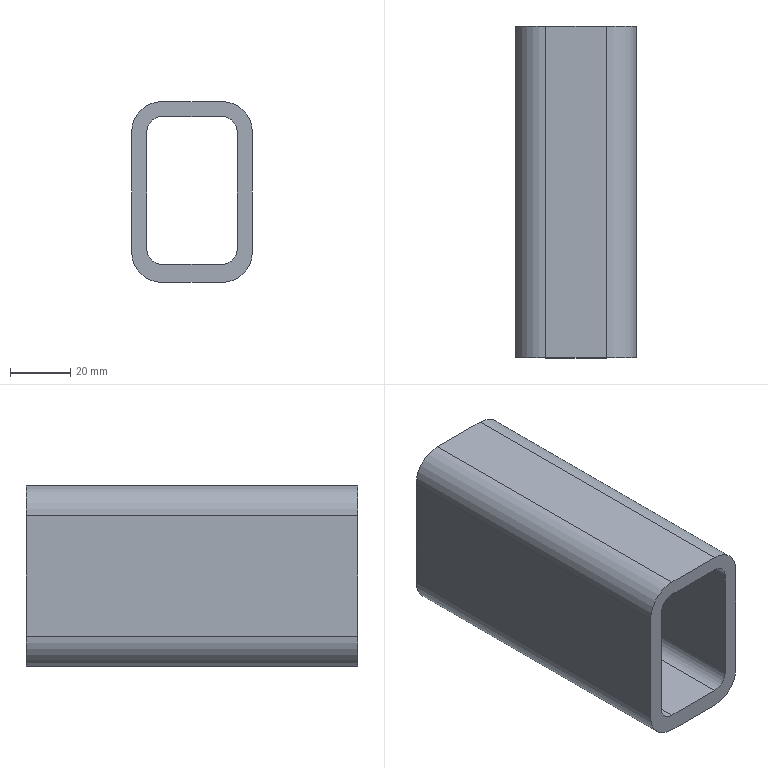Part | STEP file | frame inner longitudinal beam 2--000.001--20240926 | 1 solid | 18 faces | box 40 x 110 x 60 mm | volume 95218 mm3 | plane 10 | cylinder 8 | commonest cylinder face diameters 10 x4 20 x4
STEP:
#1=CARTESIAN_POINT('',(0.,0.,0.));
#2=DIRECTION('',(0.,0.,1.));
#3=DIRECTION('',(1.,0.,0.));
#4=AXIS2_PLACEMENT_3D('',#1,#2,#3);
#5=CARTESIAN_POINT('',(-30.,-995.,50.));
#6=VERTEX_POINT('',#5);
#7=CARTESIAN_POINT('',(-30.,-885.,50.));
#8=VERTEX_POINT('',#7);
#9=CARTESIAN_POINT('',(-30.,490.173,50.));
#10=DIRECTION('',(0.,1.,0.));
#11=VECTOR('',#10,1.);
#12=LINE('',#9,#11);
#13=CARTESIAN_POINT('',(-30.,490.173,40.));
#14=DIRECTION('',(0.,1.,0.));
#15=DIRECTION('',(0.,0.,-1.));
#16=AXIS2_PLACEMENT_3D('',#13,#14,#15);
#17=CYLINDRICAL_SURFACE('',#16,10.);
#18=CARTESIAN_POINT('',(3.142,0.));
#19=DIRECTION('',(0.,1.));
#20=VECTOR('',#19,1.);
#21=LINE('',#18,#20);
#22=(GEOMETRIC_REPRESENTATION_CONTEXT(2)PARAMETRIC_REPRESENTATION_CONTEXT()REPRESENTATION_CONTEXT('',''));
#23=DEFINITIONAL_REPRESENTATION('',(#21),#22);
#24=PCURVE('',#17,#23);
#25=CARTESIAN_POINT('',(-40.,490.173,50.));
#26=DIRECTION('',(0.,0.,-1.));
#27=DIRECTION('',(0.,-1.,0.));
#28=AXIS2_PLACEMENT_3D('',#25,#26,#27);
#29=PLANE('',#28);
#30=CARTESIAN_POINT('',(0.,-10.));
#31=DIRECTION('',(-1.,0.));
#32=VECTOR('',#31,1.);
#33=LINE('',#30,#32);
#34=(GEOMETRIC_REPRESENTATION_CONTEXT(2)PARAMETRIC_REPRESENTATION_CONTEXT()REPRESENTATION_CONTEXT('',''));
#35=DEFINITIONAL_REPRESENTATION('',(#33),#34);
#36=PCURVE('',#29,#35);
#37=SURFACE_CURVE('',#12,(#24,#36),.PCURVE_S1.);
#38=EDGE_CURVE('',#6,#8,#37,.T.);
#39=ORIENTED_EDGE('',*,*,#38,.T.);
#40=CARTESIAN_POINT('',(-40.,-885.,40.));
#41=VERTEX_POINT('',#40);
#42=CARTESIAN_POINT('',(-30.,-885.,40.));
#43=DIRECTION('',(0.,-1.,0.));
#44=DIRECTION('',(0.,0.,1.));
#45=AXIS2_PLACEMENT_3D('',#42,#43,#44);
#46=CIRCLE('',#45,10.);
#47=CARTESIAN_POINT('',(3.142,-1375.173));
#48=DIRECTION('',(-1.,0.));
#49=VECTOR('',#48,1.);
#50=LINE('',#47,#49);
#51=(GEOMETRIC_REPRESENTATION_CONTEXT(2)PARAMETRIC_REPRESENTATION_CONTEXT()REPRESENTATION_CONTEXT('',''));
#52=DEFINITIONAL_REPRESENTATION('',(#50),#51);
#53=PCURVE('',#17,#52);
#54=CARTESIAN_POINT('',(-360.,-885.,20.));
#55=DIRECTION('',(0.,1.,0.));
#56=DIRECTION('',(0.,0.,-1.));
#57=AXIS2_PLACEMENT_3D('',#54,#55,#56);
#58=PLANE('',#57);
#59=CARTESIAN_POINT('',(-30.,-330.));
#60=CARTESIAN_POINT('',(-30.,-312.679));
#61=CARTESIAN_POINT('',(-15.,-321.34));
#62=CARTESIAN_POINT('',(0.,-330.));
#63=CARTESIAN_POINT('',(-15.,-338.66));
#64=CARTESIAN_POINT('',(-30.,-347.321));
#65=CARTESIAN_POINT('',(-30.,-330.));
#66=(BOUNDED_CURVE()B_SPLINE_CURVE(2,(#59,#60,#61,#62,#63,#64,#65),.UNSPECIFIED.,.T.,.F.)B_SPLINE_CURVE_WITH_KNOTS((1,2,2,2,2,1),(-2.094,0.,2.094,4.189,6.283,8.378),.UNSPECIFIED.)CURVE()GEOMETRIC_REPRESENTATION_ITEM()RATIONAL_B_SPLINE_CURVE((1.,0.5,1.,0.5,1.,0.5,1.))REPRESENTATION_ITEM(''));
#67=(GEOMETRIC_REPRESENTATION_CONTEXT(2)PARAMETRIC_REPRESENTATION_CONTEXT()REPRESENTATION_CONTEXT('',''));
#68=DEFINITIONAL_REPRESENTATION('',(#66),#67);
#69=PCURVE('',#58,#68);
#70=SURFACE_CURVE('',#46,(#53,#69),.PCURVE_S1.);
#71=EDGE_CURVE('',#8,#41,#70,.T.);
#72=ORIENTED_EDGE('',*,*,#71,.T.);
#73=CARTESIAN_POINT('',(-40.,-995.,40.));
#74=VERTEX_POINT('',#73);
#75=CARTESIAN_POINT('',(-40.,490.173,40.));
#76=DIRECTION('',(0.,-1.,0.));
#77=VECTOR('',#76,1.);
#78=LINE('',#75,#77);
#79=CARTESIAN_POINT('',(1.571,0.));
#80=DIRECTION('',(0.,-1.));
#81=VECTOR('',#80,1.);
#82=LINE('',#79,#81);
#83=(GEOMETRIC_REPRESENTATION_CONTEXT(2)PARAMETRIC_REPRESENTATION_CONTEXT()REPRESENTATION_CONTEXT('',''));
#84=DEFINITIONAL_REPRESENTATION('',(#82),#83);
#85=PCURVE('',#17,#84);
#86=CARTESIAN_POINT('',(-40.,490.173,10.));
#87=DIRECTION('',(1.,0.,0.));
#88=DIRECTION('',(0.,0.9613,-0.2756));
#89=AXIS2_PLACEMENT_3D('',#86,#87,#88);
#90=PLANE('',#89);
#91=CARTESIAN_POINT('',(-8.269,28.838));
#92=DIRECTION('',(-0.9613,-0.2756));
#93=VECTOR('',#92,1.);
#94=LINE('',#91,#93);
#95=(GEOMETRIC_REPRESENTATION_CONTEXT(2)PARAMETRIC_REPRESENTATION_CONTEXT()REPRESENTATION_CONTEXT('',''));
#96=DEFINITIONAL_REPRESENTATION('',(#94),#95);
#97=PCURVE('',#90,#96);
#98=SURFACE_CURVE('',#78,(#85,#97),.PCURVE_S1.);
#99=EDGE_CURVE('',#41,#74,#98,.T.);
#100=ORIENTED_EDGE('',*,*,#99,.T.);
#101=CARTESIAN_POINT('',(-30.,-995.,40.));
#102=DIRECTION('',(0.,-1.,0.));
#103=DIRECTION('',(0.,0.,1.));
#104=AXIS2_PLACEMENT_3D('',#101,#102,#103);
#105=CIRCLE('',#104,10.);
#106=CARTESIAN_POINT('',(3.142,-1485.173));
#107=DIRECTION('',(-1.,0.));
#108=VECTOR('',#107,1.);
#109=LINE('',#106,#108);
#110=(GEOMETRIC_REPRESENTATION_CONTEXT(2)PARAMETRIC_REPRESENTATION_CONTEXT()REPRESENTATION_CONTEXT('',''));
#111=DEFINITIONAL_REPRESENTATION('',(#109),#110);
#112=PCURVE('',#17,#111);
#113=CARTESIAN_POINT('',(-40.,-995.,-13.42));
#114=DIRECTION('',(0.,1.,0.));
#115=DIRECTION('',(0.,0.,-1.));
#116=AXIS2_PLACEMENT_3D('',#113,#114,#115);
#117=PLANE('',#116);
#118=CARTESIAN_POINT('',(-63.42,-10.));
#119=CARTESIAN_POINT('',(-63.42,7.321));
#120=CARTESIAN_POINT('',(-48.42,-1.34));
#121=CARTESIAN_POINT('',(-33.42,-10.));
#122=CARTESIAN_POINT('',(-48.42,-18.66));
#123=CARTESIAN_POINT('',(-63.42,-27.321));
#124=CARTESIAN_POINT('',(-63.42,-10.));
#125=(BOUNDED_CURVE()B_SPLINE_CURVE(2,(#118,#119,#120,#121,#122,#123,#124),.UNSPECIFIED.,.T.,.F.)B_SPLINE_CURVE_WITH_KNOTS((1,2,2,2,2,1),(-2.094,0.,2.094,4.189,6.283,8.378),.UNSPECIFIED.)CURVE()GEOMETRIC_REPRESENTATION_ITEM()RATIONAL_B_SPLINE_CURVE((1.,0.5,1.,0.5,1.,0.5,1.))REPRESENTATION_ITEM(''));
#126=(GEOMETRIC_REPRESENTATION_CONTEXT(2)PARAMETRIC_REPRESENTATION_CONTEXT()REPRESENTATION_CONTEXT('',''));
#127=DEFINITIONAL_REPRESENTATION('',(#125),#126);
#128=PCURVE('',#117,#127);
#129=SURFACE_CURVE('',#105,(#112,#128),.PCURVE_S1.);
#130=EDGE_CURVE('',#6,#74,#129,.T.);
#131=ORIENTED_EDGE('',*,*,#130,.F.);
#132=EDGE_LOOP('',(#39,#72,#100,#131));
#133=FACE_BOUND('',#132,.T.);
#134=ADVANCED_FACE('',(#133),#17,.T.);
#135=CARTESIAN_POINT('',(-40.,-995.,0.));
#136=VERTEX_POINT('',#135);
#137=CARTESIAN_POINT('',(-40.,-885.,0.));
#138=VERTEX_POINT('',#137);
#139=CARTESIAN_POINT('',(-40.,1110.173,0.));
#140=DIRECTION('',(0.,1.,0.));
#141=VECTOR('',#140,1.);
#142=LINE('',#139,#141);
#143=CARTESIAN_POINT('',(-30.,1110.173,0.));
#144=DIRECTION('',(0.,1.,0.));
#145=DIRECTION('',(0.,0.,-1.));
#146=AXIS2_PLACEMENT_3D('',#143,#144,#145);
#147=CYLINDRICAL_SURFACE('',#146,10.);
#148=CARTESIAN_POINT('',(1.571,0.));
#149=DIRECTION('',(0.,1.));
#150=VECTOR('',#149,1.);
#151=LINE('',#148,#150);
#152=(GEOMETRIC_REPRESENTATION_CONTEXT(2)PARAMETRIC_REPRESENTATION_CONTEXT()REPRESENTATION_CONTEXT('',''));
#153=DEFINITIONAL_REPRESENTATION('',(#151),#152);
#154=PCURVE('',#147,#153);
#155=CARTESIAN_POINT('',(598.739,161.283));
#156=DIRECTION('',(0.9613,0.2756));
#157=VECTOR('',#156,1.);
#158=LINE('',#155,#157);
#159=(GEOMETRIC_REPRESENTATION_CONTEXT(2)PARAMETRIC_REPRESENTATION_CONTEXT()REPRESENTATION_CONTEXT('',''));
#160=DEFINITIONAL_REPRESENTATION('',(#158),#159);
#161=PCURVE('',#90,#160);
#162=SURFACE_CURVE('',#142,(#154,#161),.PCURVE_S1.);
#163=EDGE_CURVE('',#136,#138,#162,.T.);
#164=ORIENTED_EDGE('',*,*,#163,.T.);
#165=CARTESIAN_POINT('',(-30.,-885.,-10.));
#166=VERTEX_POINT('',#165);
#167=CARTESIAN_POINT('',(-30.,-885.,0.));
#168=DIRECTION('',(0.,-1.,0.));
#169=DIRECTION('',(0.,0.,1.));
#170=AXIS2_PLACEMENT_3D('',#167,#168,#169);
#171=CIRCLE('',#170,10.);
#172=CARTESIAN_POINT('',(3.142,-1995.173));
#173=DIRECTION('',(-1.,0.));
#174=VECTOR('',#173,1.);
#175=LINE('',#172,#174);
#176=(GEOMETRIC_REPRESENTATION_CONTEXT(2)PARAMETRIC_REPRESENTATION_CONTEXT()REPRESENTATION_CONTEXT('',''));
#177=DEFINITIONAL_REPRESENTATION('',(#175),#176);
#178=PCURVE('',#147,#177);
#179=CARTESIAN_POINT('',(10.,-330.));
#180=CARTESIAN_POINT('',(10.,-312.679));
#181=CARTESIAN_POINT('',(25.,-321.34));
#182=CARTESIAN_POINT('',(40.,-330.));
#183=CARTESIAN_POINT('',(25.,-338.66));
#184=CARTESIAN_POINT('',(10.,-347.321));
#185=CARTESIAN_POINT('',(10.,-330.));
#186=(BOUNDED_CURVE()B_SPLINE_CURVE(2,(#179,#180,#181,#182,#183,#184,#185),.UNSPECIFIED.,.T.,.F.)B_SPLINE_CURVE_WITH_KNOTS((1,2,2,2,2,1),(-2.094,0.,2.094,4.189,6.283,8.378),.UNSPECIFIED.)CURVE()GEOMETRIC_REPRESENTATION_ITEM()RATIONAL_B_SPLINE_CURVE((1.,0.5,1.,0.5,1.,0.5,1.))REPRESENTATION_ITEM(''));
#187=(GEOMETRIC_REPRESENTATION_CONTEXT(2)PARAMETRIC_REPRESENTATION_CONTEXT()REPRESENTATION_CONTEXT('',''));
#188=DEFINITIONAL_REPRESENTATION('',(#186),#187);
#189=PCURVE('',#58,#188);
#190=SURFACE_CURVE('',#171,(#178,#189),.PCURVE_S1.);
#191=EDGE_CURVE('',#138,#166,#190,.T.);
#192=ORIENTED_EDGE('',*,*,#191,.T.);
#193=CARTESIAN_POINT('',(-30.,-995.,-10.));
#194=VERTEX_POINT('',#193);
#195=CARTESIAN_POINT('',(-30.,1110.173,-10.));
#196=DIRECTION('',(0.,-1.,0.));
#197=VECTOR('',#196,1.);
#198=LINE('',#195,#197);
#199=CARTESIAN_POINT('',(0.,0.));
#200=DIRECTION('',(0.,-1.));
#201=VECTOR('',#200,1.);
#202=LINE('',#199,#201);
#203=(GEOMETRIC_REPRESENTATION_CONTEXT(2)PARAMETRIC_REPRESENTATION_CONTEXT()REPRESENTATION_CONTEXT('',''));
#204=DEFINITIONAL_REPRESENTATION('',(#202),#203);
#205=PCURVE('',#147,#204);
#206=CARTESIAN_POINT('',(0.,1110.173,-10.));
#207=DIRECTION('',(0.,0.,1.));
#208=DIRECTION('',(0.,1.,0.));
#209=AXIS2_PLACEMENT_3D('',#206,#207,#208);
#210=PLANE('',#209);
#211=CARTESIAN_POINT('',(0.,30.));
#212=DIRECTION('',(-1.,0.));
#213=VECTOR('',#212,1.);
#214=LINE('',#211,#213);
#215=(GEOMETRIC_REPRESENTATION_CONTEXT(2)PARAMETRIC_REPRESENTATION_CONTEXT()REPRESENTATION_CONTEXT('',''));
#216=DEFINITIONAL_REPRESENTATION('',(#214),#215);
#217=PCURVE('',#210,#216);
#218=SURFACE_CURVE('',#198,(#205,#217),.PCURVE_S1.);
#219=EDGE_CURVE('',#166,#194,#218,.T.);
#220=ORIENTED_EDGE('',*,*,#219,.T.);
#221=CARTESIAN_POINT('',(-30.,-995.,0.));
#222=DIRECTION('',(0.,-1.,0.));
#223=DIRECTION('',(0.,0.,1.));
#224=AXIS2_PLACEMENT_3D('',#221,#222,#223);
#225=CIRCLE('',#224,10.);
#226=CARTESIAN_POINT('',(3.142,-2105.173));
#227=DIRECTION('',(-1.,0.));
#228=VECTOR('',#227,1.);
#229=LINE('',#226,#228);
#230=(GEOMETRIC_REPRESENTATION_CONTEXT(2)PARAMETRIC_REPRESENTATION_CONTEXT()REPRESENTATION_CONTEXT('',''));
#231=DEFINITIONAL_REPRESENTATION('',(#229),#230);
#232=PCURVE('',#147,#231);
#233=CARTESIAN_POINT('',(-23.42,-10.));
#234=CARTESIAN_POINT('',(-23.42,7.321));
#235=CARTESIAN_POINT('',(-8.42,-1.34));
#236=CARTESIAN_POINT('',(6.58,-10.));
#237=CARTESIAN_POINT('',(-8.42,-18.66));
#238=CARTESIAN_POINT('',(-23.42,-27.321));
#239=CARTESIAN_POINT('',(-23.42,-10.));
#240=(BOUNDED_CURVE()B_SPLINE_CURVE(2,(#233,#234,#235,#236,#237,#238,#239),.UNSPECIFIED.,.T.,.F.)B_SPLINE_CURVE_WITH_KNOTS((1,2,2,2,2,1),(-2.094,0.,2.094,4.189,6.283,8.378),.UNSPECIFIED.)CURVE()GEOMETRIC_REPRESENTATION_ITEM()RATIONAL_B_SPLINE_CURVE((1.,0.5,1.,0.5,1.,0.5,1.))REPRESENTATION_ITEM(''));
#241=(GEOMETRIC_REPRESENTATION_CONTEXT(2)PARAMETRIC_REPRESENTATION_CONTEXT()REPRESENTATION_CONTEXT('',''));
#242=DEFINITIONAL_REPRESENTATION('',(#240),#241);
#243=PCURVE('',#117,#242);
#244=SURFACE_CURVE('',#225,(#232,#243),.PCURVE_S1.);
#245=EDGE_CURVE('',#136,#194,#244,.T.);
#246=ORIENTED_EDGE('',*,*,#245,.F.);
#247=EDGE_LOOP('',(#164,#192,#220,#246));
#248=FACE_BOUND('',#247,.T.);
#249=ADVANCED_FACE('',(#248),#147,.T.);
#250=CARTESIAN_POINT('',(-40.,-885.,10.));
#251=DIRECTION('',(0.,0.,1.));
#252=VECTOR('',#251,1.);
#253=LINE('',#250,#252);
#254=CARTESIAN_POINT('',(-1321.901,-379.049));
#255=DIRECTION('',(-0.2756,0.9613));
#256=VECTOR('',#255,1.);
#257=LINE('',#254,#256);
#258=(GEOMETRIC_REPRESENTATION_CONTEXT(2)PARAMETRIC_REPRESENTATION_CONTEXT()REPRESENTATION_CONTEXT('',''));
#259=DEFINITIONAL_REPRESENTATION('',(#257),#258);
#260=PCURVE('',#90,#259);
#261=CARTESIAN_POINT('',(10.,-320.));
#262=DIRECTION('',(-1.,0.));
#263=VECTOR('',#262,1.);
#264=LINE('',#261,#263);
#265=(GEOMETRIC_REPRESENTATION_CONTEXT(2)PARAMETRIC_REPRESENTATION_CONTEXT()REPRESENTATION_CONTEXT('',''));
#266=DEFINITIONAL_REPRESENTATION('',(#264),#265);
#267=PCURVE('',#58,#266);
#268=SURFACE_CURVE('',#253,(#260,#267),.PCURVE_S1.);
#269=EDGE_CURVE('',#138,#41,#268,.T.);
#270=ORIENTED_EDGE('',*,*,#269,.F.);
#271=ORIENTED_EDGE('',*,*,#163,.F.);
#272=CARTESIAN_POINT('',(-40.,-995.,10.));
#273=DIRECTION('',(0.,0.,1.));
#274=VECTOR('',#273,1.);
#275=LINE('',#272,#274);
#276=CARTESIAN_POINT('',(-1427.64,-409.369));
#277=DIRECTION('',(-0.2756,0.9613));
#278=VECTOR('',#277,1.);
#279=LINE('',#276,#278);
#280=(GEOMETRIC_REPRESENTATION_CONTEXT(2)PARAMETRIC_REPRESENTATION_CONTEXT()REPRESENTATION_CONTEXT('',''));
#281=DEFINITIONAL_REPRESENTATION('',(#279),#280);
#282=PCURVE('',#90,#281);
#283=CARTESIAN_POINT('',(-23.42,0.));
#284=DIRECTION('',(-1.,0.));
#285=VECTOR('',#284,1.);
#286=LINE('',#283,#285);
#287=(GEOMETRIC_REPRESENTATION_CONTEXT(2)PARAMETRIC_REPRESENTATION_CONTEXT()REPRESENTATION_CONTEXT('',''));
#288=DEFINITIONAL_REPRESENTATION('',(#286),#287);
#289=PCURVE('',#117,#288);
#290=SURFACE_CURVE('',#275,(#282,#289),.PCURVE_S1.);
#291=EDGE_CURVE('',#136,#74,#290,.T.);
#292=ORIENTED_EDGE('',*,*,#291,.T.);
#293=ORIENTED_EDGE('',*,*,#99,.F.);
#294=EDGE_LOOP('',(#270,#271,#292,#293));
#295=FACE_BOUND('',#294,.T.);
#296=ADVANCED_FACE('',(#295),#90,.F.);
#297=CARTESIAN_POINT('',(-10.,-995.,-10.));
#298=VERTEX_POINT('',#297);
#299=CARTESIAN_POINT('',(-10.,-885.,-10.));
#300=VERTEX_POINT('',#299);
#301=CARTESIAN_POINT('',(-10.,490.173,-10.));
#302=DIRECTION('',(0.,1.,0.));
#303=VECTOR('',#302,1.);
#304=LINE('',#301,#303);
#305=CARTESIAN_POINT('',(-10.,490.173,0.));
#306=DIRECTION('',(0.,1.,0.));
#307=DIRECTION('',(0.,0.,-1.));
#308=AXIS2_PLACEMENT_3D('',#305,#306,#307);
#309=CYLINDRICAL_SURFACE('',#308,10.);
#310=CARTESIAN_POINT('',(6.283,0.));
#311=DIRECTION('',(0.,1.));
#312=VECTOR('',#311,1.);
#313=LINE('',#310,#312);
#314=(GEOMETRIC_REPRESENTATION_CONTEXT(2)PARAMETRIC_REPRESENTATION_CONTEXT()REPRESENTATION_CONTEXT('',''));
#315=DEFINITIONAL_REPRESENTATION('',(#313),#314);
#316=PCURVE('',#309,#315);
#317=CARTESIAN_POINT('',(-620.,10.));
#318=DIRECTION('',(1.,0.));
#319=VECTOR('',#318,1.);
#320=LINE('',#317,#319);
#321=(GEOMETRIC_REPRESENTATION_CONTEXT(2)PARAMETRIC_REPRESENTATION_CONTEXT()REPRESENTATION_CONTEXT('',''));
#322=DEFINITIONAL_REPRESENTATION('',(#320),#321);
#323=PCURVE('',#210,#322);
#324=SURFACE_CURVE('',#304,(#316,#323),.PCURVE_S1.);
#325=EDGE_CURVE('',#298,#300,#324,.T.);
#326=ORIENTED_EDGE('',*,*,#325,.T.);
#327=CARTESIAN_POINT('',(0.,-885.,0.));
#328=VERTEX_POINT('',#327);
#329=CARTESIAN_POINT('',(-10.,-885.,0.));
#330=DIRECTION('',(0.,-1.,0.));
#331=DIRECTION('',(0.,0.,1.));
#332=AXIS2_PLACEMENT_3D('',#329,#330,#331);
#333=CIRCLE('',#332,10.);
#334=CARTESIAN_POINT('',(9.425,-1375.173));
#335=DIRECTION('',(-1.,0.));
#336=VECTOR('',#335,1.);
#337=LINE('',#334,#336);
#338=(GEOMETRIC_REPRESENTATION_CONTEXT(2)PARAMETRIC_REPRESENTATION_CONTEXT()REPRESENTATION_CONTEXT('',''));
#339=DEFINITIONAL_REPRESENTATION('',(#337),#338);
#340=PCURVE('',#309,#339);
#341=CARTESIAN_POINT('',(10.,-350.));
#342=CARTESIAN_POINT('',(10.,-332.679));
#343=CARTESIAN_POINT('',(25.,-341.34));
#344=CARTESIAN_POINT('',(40.,-350.));
#345=CARTESIAN_POINT('',(25.,-358.66));
#346=CARTESIAN_POINT('',(10.,-367.321));
#347=CARTESIAN_POINT('',(10.,-350.));
#348=(BOUNDED_CURVE()B_SPLINE_CURVE(2,(#341,#342,#343,#344,#345,#346,#347),.UNSPECIFIED.,.T.,.F.)B_SPLINE_CURVE_WITH_KNOTS((1,2,2,2,2,1),(-2.094,0.,2.094,4.189,6.283,8.378),.UNSPECIFIED.)CURVE()GEOMETRIC_REPRESENTATION_ITEM()RATIONAL_B_SPLINE_CURVE((1.,0.5,1.,0.5,1.,0.5,1.))REPRESENTATION_ITEM(''));
#349=(GEOMETRIC_REPRESENTATION_CONTEXT(2)PARAMETRIC_REPRESENTATION_CONTEXT()REPRESENTATION_CONTEXT('',''));
#350=DEFINITIONAL_REPRESENTATION('',(#348),#349);
#351=PCURVE('',#58,#350);
#352=SURFACE_CURVE('',#333,(#340,#351),.PCURVE_S1.);
#353=EDGE_CURVE('',#300,#328,#352,.T.);
#354=ORIENTED_EDGE('',*,*,#353,.T.);
#355=CARTESIAN_POINT('',(0.,-995.,0.));
#356=VERTEX_POINT('',#355);
#357=CARTESIAN_POINT('',(0.,490.173,0.));
#358=DIRECTION('',(0.,-1.,0.));
#359=VECTOR('',#358,1.);
#360=LINE('',#357,#359);
#361=CARTESIAN_POINT('',(4.712,0.));
#362=DIRECTION('',(0.,-1.));
#363=VECTOR('',#362,1.);
#364=LINE('',#361,#363);
#365=(GEOMETRIC_REPRESENTATION_CONTEXT(2)PARAMETRIC_REPRESENTATION_CONTEXT()REPRESENTATION_CONTEXT('',''));
#366=DEFINITIONAL_REPRESENTATION('',(#364),#365);
#367=PCURVE('',#309,#366);
#368=CARTESIAN_POINT('',(0.,490.173,50.));
#369=DIRECTION('',(-1.,0.,0.));
#370=DIRECTION('',(0.,-0.9613,0.2756));
#371=AXIS2_PLACEMENT_3D('',#368,#369,#370);
#372=PLANE('',#371);
#373=CARTESIAN_POINT('',(-13.782,-48.063));
#374=DIRECTION('',(0.9613,-0.2756));
#375=VECTOR('',#374,1.);
#376=LINE('',#373,#375);
#377=(GEOMETRIC_REPRESENTATION_CONTEXT(2)PARAMETRIC_REPRESENTATION_CONTEXT()REPRESENTATION_CONTEXT('',''));
#378=DEFINITIONAL_REPRESENTATION('',(#376),#377);
#379=PCURVE('',#372,#378);
#380=SURFACE_CURVE('',#360,(#367,#379),.PCURVE_S1.);
#381=EDGE_CURVE('',#328,#356,#380,.T.);
#382=ORIENTED_EDGE('',*,*,#381,.T.);
#383=CARTESIAN_POINT('',(-10.,-995.,0.));
#384=DIRECTION('',(0.,1.,0.));
#385=DIRECTION('',(0.,0.,1.));
#386=AXIS2_PLACEMENT_3D('',#383,#384,#385);
#387=CIRCLE('',#386,10.);
#388=CARTESIAN_POINT('',(3.142,-1485.173));
#389=DIRECTION('',(1.,0.));
#390=VECTOR('',#389,1.);
#391=LINE('',#388,#390);
#392=(GEOMETRIC_REPRESENTATION_CONTEXT(2)PARAMETRIC_REPRESENTATION_CONTEXT()REPRESENTATION_CONTEXT('',''));
#393=DEFINITIONAL_REPRESENTATION('',(#391),#392);
#394=PCURVE('',#309,#393);
#395=CARTESIAN_POINT('',(-13.42,-30.));
#396=DIRECTION('',(-1.,0.));
#397=AXIS2_PLACEMENT_2D('',#395,#396);
#398=CIRCLE('',#397,10.);
#399=(GEOMETRIC_REPRESENTATION_CONTEXT(2)PARAMETRIC_REPRESENTATION_CONTEXT()REPRESENTATION_CONTEXT('',''));
#400=DEFINITIONAL_REPRESENTATION('',(#398),#399);
#401=PCURVE('',#117,#400);
#402=SURFACE_CURVE('',#387,(#394,#401),.PCURVE_S1.);
#403=EDGE_CURVE('',#356,#298,#402,.T.);
#404=ORIENTED_EDGE('',*,*,#403,.T.);
#405=EDGE_LOOP('',(#326,#354,#382,#404));
#406=FACE_BOUND('',#405,.T.);
#407=ADVANCED_FACE('',(#406),#309,.T.);
#408=CARTESIAN_POINT('',(0.,-885.,-10.));
#409=DIRECTION('',(-1.,0.,0.));
#410=VECTOR('',#409,1.);
#411=LINE('',#408,#410);
#412=CARTESIAN_POINT('',(-1995.173,0.));
#413=DIRECTION('',(0.,1.));
#414=VECTOR('',#413,1.);
#415=LINE('',#412,#414);
#416=(GEOMETRIC_REPRESENTATION_CONTEXT(2)PARAMETRIC_REPRESENTATION_CONTEXT()REPRESENTATION_CONTEXT('',''));
#417=DEFINITIONAL_REPRESENTATION('',(#415),#416);
#418=PCURVE('',#210,#417);
#419=CARTESIAN_POINT('',(30.,-360.));
#420=DIRECTION('',(0.,1.));
#421=VECTOR('',#420,1.);
#422=LINE('',#419,#421);
#423=(GEOMETRIC_REPRESENTATION_CONTEXT(2)PARAMETRIC_REPRESENTATION_CONTEXT()REPRESENTATION_CONTEXT('',''));
#424=DEFINITIONAL_REPRESENTATION('',(#422),#423);
#425=PCURVE('',#58,#424);
#426=SURFACE_CURVE('',#411,(#418,#425),.PCURVE_S1.);
#427=EDGE_CURVE('',#300,#166,#426,.T.);
#428=ORIENTED_EDGE('',*,*,#427,.F.);
#429=ORIENTED_EDGE('',*,*,#325,.F.);
#430=CARTESIAN_POINT('',(-40.,-995.,-10.));
#431=DIRECTION('',(1.,0.,0.));
#432=VECTOR('',#431,1.);
#433=LINE('',#430,#432);
#434=CARTESIAN_POINT('',(-2105.173,40.));
#435=DIRECTION('',(0.,-1.));
#436=VECTOR('',#435,1.);
#437=LINE('',#434,#436);
#438=(GEOMETRIC_REPRESENTATION_CONTEXT(2)PARAMETRIC_REPRESENTATION_CONTEXT()REPRESENTATION_CONTEXT('',''));
#439=DEFINITIONAL_REPRESENTATION('',(#437),#438);
#440=PCURVE('',#210,#439);
#441=CARTESIAN_POINT('',(-3.42,0.));
#442=DIRECTION('',(0.,-1.));
#443=VECTOR('',#442,1.);
#444=LINE('',#441,#443);
#445=(GEOMETRIC_REPRESENTATION_CONTEXT(2)PARAMETRIC_REPRESENTATION_CONTEXT()REPRESENTATION_CONTEXT('',''));
#446=DEFINITIONAL_REPRESENTATION('',(#444),#445);
#447=PCURVE('',#117,#446);
#448=SURFACE_CURVE('',#433,(#440,#447),.PCURVE_S1.);
#449=EDGE_CURVE('',#194,#298,#448,.T.);
#450=ORIENTED_EDGE('',*,*,#449,.F.);
#451=ORIENTED_EDGE('',*,*,#219,.F.);
#452=EDGE_LOOP('',(#428,#429,#450,#451));
#453=FACE_BOUND('',#452,.T.);
#454=ADVANCED_FACE('',(#453),#210,.F.);
#455=CARTESIAN_POINT('',(0.,-995.,40.));
#456=VERTEX_POINT('',#455);
#457=CARTESIAN_POINT('',(0.,-885.,40.));
#458=VERTEX_POINT('',#457);
#459=CARTESIAN_POINT('',(0.,490.173,40.));
#460=DIRECTION('',(0.,1.,0.));
#461=VECTOR('',#460,1.);
#462=LINE('',#459,#461);
#463=CARTESIAN_POINT('',(-10.,490.173,40.));
#464=DIRECTION('',(0.,1.,0.));
#465=DIRECTION('',(0.,0.,-1.));
#466=AXIS2_PLACEMENT_3D('',#463,#464,#465);
#467=CYLINDRICAL_SURFACE('',#466,10.);
#468=CARTESIAN_POINT('',(4.712,0.));
#469=DIRECTION('',(0.,1.));
#470=VECTOR('',#469,1.);
#471=LINE('',#468,#470);
#472=(GEOMETRIC_REPRESENTATION_CONTEXT(2)PARAMETRIC_REPRESENTATION_CONTEXT()REPRESENTATION_CONTEXT('',''));
#473=DEFINITIONAL_REPRESENTATION('',(#471),#472);
#474=PCURVE('',#467,#473);
#475=CARTESIAN_POINT('',(-2.756,-9.613));
#476=DIRECTION('',(-0.9613,0.2756));
#477=VECTOR('',#476,1.);
#478=LINE('',#475,#477);
#479=(GEOMETRIC_REPRESENTATION_CONTEXT(2)PARAMETRIC_REPRESENTATION_CONTEXT()REPRESENTATION_CONTEXT('',''));
#480=DEFINITIONAL_REPRESENTATION('',(#478),#479);
#481=PCURVE('',#372,#480);
#482=SURFACE_CURVE('',#462,(#474,#481),.PCURVE_S1.);
#483=EDGE_CURVE('',#456,#458,#482,.T.);
#484=ORIENTED_EDGE('',*,*,#483,.T.);
#485=CARTESIAN_POINT('',(-10.,-885.,50.));
#486=VERTEX_POINT('',#485);
#487=CARTESIAN_POINT('',(-10.,-885.,40.));
#488=DIRECTION('',(0.,-1.,0.));
#489=DIRECTION('',(0.,0.,1.));
#490=AXIS2_PLACEMENT_3D('',#487,#488,#489);
#491=CIRCLE('',#490,10.);
#492=CARTESIAN_POINT('',(9.425,-1375.173));
#493=DIRECTION('',(-1.,0.));
#494=VECTOR('',#493,1.);
#495=LINE('',#492,#494);
#496=(GEOMETRIC_REPRESENTATION_CONTEXT(2)PARAMETRIC_REPRESENTATION_CONTEXT()REPRESENTATION_CONTEXT('',''));
#497=DEFINITIONAL_REPRESENTATION('',(#495),#496);
#498=PCURVE('',#467,#497);
#499=CARTESIAN_POINT('',(-30.,-350.));
#500=CARTESIAN_POINT('',(-30.,-332.679));
#501=CARTESIAN_POINT('',(-15.,-341.34));
#502=CARTESIAN_POINT('',(0.,-350.));
#503=CARTESIAN_POINT('',(-15.,-358.66));
#504=CARTESIAN_POINT('',(-30.,-367.321));
#505=CARTESIAN_POINT('',(-30.,-350.));
#506=(BOUNDED_CURVE()B_SPLINE_CURVE(2,(#499,#500,#501,#502,#503,#504,#505),.UNSPECIFIED.,.T.,.F.)B_SPLINE_CURVE_WITH_KNOTS((1,2,2,2,2,1),(-2.094,0.,2.094,4.189,6.283,8.378),.UNSPECIFIED.)CURVE()GEOMETRIC_REPRESENTATION_ITEM()RATIONAL_B_SPLINE_CURVE((1.,0.5,1.,0.5,1.,0.5,1.))REPRESENTATION_ITEM(''));
#507=(GEOMETRIC_REPRESENTATION_CONTEXT(2)PARAMETRIC_REPRESENTATION_CONTEXT()REPRESENTATION_CONTEXT('',''));
#508=DEFINITIONAL_REPRESENTATION('',(#506),#507);
#509=PCURVE('',#58,#508);
#510=SURFACE_CURVE('',#491,(#498,#509),.PCURVE_S1.);
#511=EDGE_CURVE('',#458,#486,#510,.T.);
#512=ORIENTED_EDGE('',*,*,#511,.T.);
#513=CARTESIAN_POINT('',(-10.,-995.,50.));
#514=VERTEX_POINT('',#513);
#515=CARTESIAN_POINT('',(-10.,490.173,50.));
#516=DIRECTION('',(0.,-1.,0.));
#517=VECTOR('',#516,1.);
#518=LINE('',#515,#517);
#519=CARTESIAN_POINT('',(3.142,0.));
#520=DIRECTION('',(0.,-1.));
#521=VECTOR('',#520,1.);
#522=LINE('',#519,#521);
#523=(GEOMETRIC_REPRESENTATION_CONTEXT(2)PARAMETRIC_REPRESENTATION_CONTEXT()REPRESENTATION_CONTEXT('',''));
#524=DEFINITIONAL_REPRESENTATION('',(#522),#523);
#525=PCURVE('',#467,#524);
#526=CARTESIAN_POINT('',(0.,-30.));
#527=DIRECTION('',(1.,0.));
#528=VECTOR('',#527,1.);
#529=LINE('',#526,#528);
#530=(GEOMETRIC_REPRESENTATION_CONTEXT(2)PARAMETRIC_REPRESENTATION_CONTEXT()REPRESENTATION_CONTEXT('',''));
#531=DEFINITIONAL_REPRESENTATION('',(#529),#530);
#532=PCURVE('',#29,#531);
#533=SURFACE_CURVE('',#518,(#525,#532),.PCURVE_S1.);
#534=EDGE_CURVE('',#486,#514,#533,.T.);
#535=ORIENTED_EDGE('',*,*,#534,.T.);
#536=CARTESIAN_POINT('',(-10.,-995.,40.));
#537=DIRECTION('',(0.,-1.,0.));
#538=DIRECTION('',(0.,0.,1.));
#539=AXIS2_PLACEMENT_3D('',#536,#537,#538);
#540=CIRCLE('',#539,10.);
#541=CARTESIAN_POINT('',(9.425,-1485.173));
#542=DIRECTION('',(-1.,0.));
#543=VECTOR('',#542,1.);
#544=LINE('',#541,#543);
#545=(GEOMETRIC_REPRESENTATION_CONTEXT(2)PARAMETRIC_REPRESENTATION_CONTEXT()REPRESENTATION_CONTEXT('',''));
#546=DEFINITIONAL_REPRESENTATION('',(#544),#545);
#547=PCURVE('',#467,#546);
#548=CARTESIAN_POINT('',(-63.42,-30.));
#549=CARTESIAN_POINT('',(-63.42,-12.679));
#550=CARTESIAN_POINT('',(-48.42,-21.34));
#551=CARTESIAN_POINT('',(-33.42,-30.));
#552=CARTESIAN_POINT('',(-48.42,-38.66));
#553=CARTESIAN_POINT('',(-63.42,-47.321));
#554=CARTESIAN_POINT('',(-63.42,-30.));
#555=(BOUNDED_CURVE()B_SPLINE_CURVE(2,(#548,#549,#550,#551,#552,#553,#554),.UNSPECIFIED.,.T.,.F.)B_SPLINE_CURVE_WITH_KNOTS((1,2,2,2,2,1),(-2.094,0.,2.094,4.189,6.283,8.378),.UNSPECIFIED.)CURVE()GEOMETRIC_REPRESENTATION_ITEM()RATIONAL_B_SPLINE_CURVE((1.,0.5,1.,0.5,1.,0.5,1.))REPRESENTATION_ITEM(''));
#556=(GEOMETRIC_REPRESENTATION_CONTEXT(2)PARAMETRIC_REPRESENTATION_CONTEXT()REPRESENTATION_CONTEXT('',''));
#557=DEFINITIONAL_REPRESENTATION('',(#555),#556);
#558=PCURVE('',#117,#557);
#559=SURFACE_CURVE('',#540,(#547,#558),.PCURVE_S1.);
#560=EDGE_CURVE('',#456,#514,#559,.T.);
#561=ORIENTED_EDGE('',*,*,#560,.F.);
#562=EDGE_LOOP('',(#484,#512,#535,#561));
#563=FACE_BOUND('',#562,.T.);
#564=ADVANCED_FACE('',(#563),#467,.T.);
#565=CARTESIAN_POINT('',(0.,-885.,50.));
#566=DIRECTION('',(0.,0.,-1.));
#567=VECTOR('',#566,1.);
#568=LINE('',#565,#567);
#569=CARTESIAN_POINT('',(1321.901,-379.049));
#570=DIRECTION('',(-0.2756,-0.9613));
#571=VECTOR('',#570,1.);
#572=LINE('',#569,#571);
#573=(GEOMETRIC_REPRESENTATION_CONTEXT(2)PARAMETRIC_REPRESENTATION_CONTEXT()REPRESENTATION_CONTEXT('',''));
#574=DEFINITIONAL_REPRESENTATION('',(#572),#573);
#575=PCURVE('',#372,#574);
#576=CARTESIAN_POINT('',(-30.,-360.));
#577=DIRECTION('',(1.,0.));
#578=VECTOR('',#577,1.);
#579=LINE('',#576,#578);
#580=(GEOMETRIC_REPRESENTATION_CONTEXT(2)PARAMETRIC_REPRESENTATION_CONTEXT()REPRESENTATION_CONTEXT('',''));
#581=DEFINITIONAL_REPRESENTATION('',(#579),#580);
#582=PCURVE('',#58,#581);
#583=SURFACE_CURVE('',#568,(#575,#582),.PCURVE_S1.);
#584=EDGE_CURVE('',#458,#328,#583,.T.);
#585=ORIENTED_EDGE('',*,*,#584,.F.);
#586=ORIENTED_EDGE('',*,*,#483,.F.);
#587=CARTESIAN_POINT('',(0.,-995.,50.));
#588=DIRECTION('',(0.,0.,-1.));
#589=VECTOR('',#588,1.);
#590=LINE('',#587,#589);
#591=CARTESIAN_POINT('',(1427.64,-409.369));
#592=DIRECTION('',(-0.2756,-0.9613));
#593=VECTOR('',#592,1.);
#594=LINE('',#591,#593);
#595=(GEOMETRIC_REPRESENTATION_CONTEXT(2)PARAMETRIC_REPRESENTATION_CONTEXT()REPRESENTATION_CONTEXT('',''));
#596=DEFINITIONAL_REPRESENTATION('',(#594),#595);
#597=PCURVE('',#372,#596);
#598=CARTESIAN_POINT('',(-63.42,-40.));
#599=DIRECTION('',(1.,0.));
#600=VECTOR('',#599,1.);
#601=LINE('',#598,#600);
#602=(GEOMETRIC_REPRESENTATION_CONTEXT(2)PARAMETRIC_REPRESENTATION_CONTEXT()REPRESENTATION_CONTEXT('',''));
#603=DEFINITIONAL_REPRESENTATION('',(#601),#602);
#604=PCURVE('',#117,#603);
#605=SURFACE_CURVE('',#590,(#597,#604),.PCURVE_S1.);
#606=EDGE_CURVE('',#456,#356,#605,.T.);
#607=ORIENTED_EDGE('',*,*,#606,.T.);
#608=ORIENTED_EDGE('',*,*,#381,.F.);
#609=EDGE_LOOP('',(#585,#586,#607,#608));
#610=FACE_BOUND('',#609,.T.);
#611=ADVANCED_FACE('',(#610),#372,.F.);
#612=CARTESIAN_POINT('',(-40.,-885.,50.));
#613=DIRECTION('',(1.,0.,0.));
#614=VECTOR('',#613,1.);
#615=LINE('',#612,#614);
#616=CARTESIAN_POINT('',(1375.173,0.));
#617=DIRECTION('',(0.,-1.));
#618=VECTOR('',#617,1.);
#619=LINE('',#616,#618);
#620=(GEOMETRIC_REPRESENTATION_CONTEXT(2)PARAMETRIC_REPRESENTATION_CONTEXT()REPRESENTATION_CONTEXT('',''));
#621=DEFINITIONAL_REPRESENTATION('',(#619),#620);
#622=PCURVE('',#29,#621);
#623=CARTESIAN_POINT('',(-30.,-320.));
#624=DIRECTION('',(0.,-1.));
#625=VECTOR('',#624,1.);
#626=LINE('',#623,#625);
#627=(GEOMETRIC_REPRESENTATION_CONTEXT(2)PARAMETRIC_REPRESENTATION_CONTEXT()REPRESENTATION_CONTEXT('',''));
#628=DEFINITIONAL_REPRESENTATION('',(#626),#627);
#629=PCURVE('',#58,#628);
#630=SURFACE_CURVE('',#615,(#622,#629),.PCURVE_S1.);
#631=EDGE_CURVE('',#8,#486,#630,.T.);
#632=ORIENTED_EDGE('',*,*,#631,.F.);
#633=ORIENTED_EDGE('',*,*,#38,.F.);
#634=CARTESIAN_POINT('',(-40.,-995.,50.));
#635=DIRECTION('',(1.,0.,0.));
#636=VECTOR('',#635,1.);
#637=LINE('',#634,#636);
#638=CARTESIAN_POINT('',(1485.173,0.));
#639=DIRECTION('',(0.,-1.));
#640=VECTOR('',#639,1.);
#641=LINE('',#638,#640);
#642=(GEOMETRIC_REPRESENTATION_CONTEXT(2)PARAMETRIC_REPRESENTATION_CONTEXT()REPRESENTATION_CONTEXT('',''));
#643=DEFINITIONAL_REPRESENTATION('',(#641),#642);
#644=PCURVE('',#29,#643);
#645=CARTESIAN_POINT('',(-63.42,0.));
#646=DIRECTION('',(0.,-1.));
#647=VECTOR('',#646,1.);
#648=LINE('',#645,#647);
#649=(GEOMETRIC_REPRESENTATION_CONTEXT(2)PARAMETRIC_REPRESENTATION_CONTEXT()REPRESENTATION_CONTEXT('',''));
#650=DEFINITIONAL_REPRESENTATION('',(#648),#649);
#651=PCURVE('',#117,#650);
#652=SURFACE_CURVE('',#637,(#644,#651),.PCURVE_S1.);
#653=EDGE_CURVE('',#6,#514,#652,.T.);
#654=ORIENTED_EDGE('',*,*,#653,.T.);
#655=ORIENTED_EDGE('',*,*,#534,.F.);
#656=EDGE_LOOP('',(#632,#633,#654,#655));
#657=FACE_BOUND('',#656,.T.);
#658=ADVANCED_FACE('',(#657),#29,.F.);
#659=CARTESIAN_POINT('',(-10.,-885.,45.));
#660=VERTEX_POINT('',#659);
#661=CARTESIAN_POINT('',(-10.,-995.,45.));
#662=VERTEX_POINT('',#661);
#663=CARTESIAN_POINT('',(-10.,-1963.827,45.));
#664=DIRECTION('',(0.,-1.,0.));
#665=VECTOR('',#664,1.);
#666=LINE('',#663,#665);
#667=CARTESIAN_POINT('',(-10.,490.173,40.));
#668=DIRECTION('',(0.,-1.,0.));
#669=DIRECTION('',(0.,0.,1.));
#670=AXIS2_PLACEMENT_3D('',#667,#668,#669);
#671=CYLINDRICAL_SURFACE('',#670,5.);
#672=CARTESIAN_POINT('',(6.283,2454.));
#673=DIRECTION('',(0.,1.));
#674=VECTOR('',#673,1.);
#675=LINE('',#672,#674);
#676=(GEOMETRIC_REPRESENTATION_CONTEXT(2)PARAMETRIC_REPRESENTATION_CONTEXT()REPRESENTATION_CONTEXT('',''));
#677=DEFINITIONAL_REPRESENTATION('',(#675),#676);
#678=PCURVE('',#671,#677);
#679=CARTESIAN_POINT('',(-2.,490.173,45.));
#680=DIRECTION('',(0.,0.,1.));
#681=DIRECTION('',(0.,1.,0.));
#682=AXIS2_PLACEMENT_3D('',#679,#680,#681);
#683=PLANE('',#682);
#684=CARTESIAN_POINT('',(-2454.,8.));
#685=DIRECTION('',(-1.,0.));
#686=VECTOR('',#685,1.);
#687=LINE('',#684,#686);
#688=(GEOMETRIC_REPRESENTATION_CONTEXT(2)PARAMETRIC_REPRESENTATION_CONTEXT()REPRESENTATION_CONTEXT('',''));
#689=DEFINITIONAL_REPRESENTATION('',(#687),#688);
#690=PCURVE('',#683,#689);
#691=SURFACE_CURVE('',#666,(#678,#690),.PCURVE_S1.);
#692=EDGE_CURVE('',#660,#662,#691,.T.);
#693=ORIENTED_EDGE('',*,*,#692,.T.);
#694=CARTESIAN_POINT('',(-5.,-995.,40.));
#695=VERTEX_POINT('',#694);
#696=CARTESIAN_POINT('',(-10.,-995.,40.));
#697=DIRECTION('',(0.,-1.,0.));
#698=DIRECTION('',(0.,0.,1.));
#699=AXIS2_PLACEMENT_3D('',#696,#697,#698);
#700=CIRCLE('',#699,5.);
#701=CARTESIAN_POINT('',(0.,1485.173));
#702=DIRECTION('',(1.,0.));
#703=VECTOR('',#702,1.);
#704=LINE('',#701,#703);
#705=(GEOMETRIC_REPRESENTATION_CONTEXT(2)PARAMETRIC_REPRESENTATION_CONTEXT()REPRESENTATION_CONTEXT('',''));
#706=DEFINITIONAL_REPRESENTATION('',(#704),#705);
#707=PCURVE('',#671,#706);
#708=CARTESIAN_POINT('',(-58.42,-30.));
#709=CARTESIAN_POINT('',(-58.42,-21.34));
#710=CARTESIAN_POINT('',(-50.92,-25.67));
#711=CARTESIAN_POINT('',(-43.42,-30.));
#712=CARTESIAN_POINT('',(-50.92,-34.33));
#713=CARTESIAN_POINT('',(-58.42,-38.66));
#714=CARTESIAN_POINT('',(-58.42,-30.));
#715=(BOUNDED_CURVE()B_SPLINE_CURVE(2,(#708,#709,#710,#711,#712,#713,#714),.UNSPECIFIED.,.T.,.F.)B_SPLINE_CURVE_WITH_KNOTS((1,2,2,2,2,1),(-2.094,0.,2.094,4.189,6.283,8.378),.UNSPECIFIED.)CURVE()GEOMETRIC_REPRESENTATION_ITEM()RATIONAL_B_SPLINE_CURVE((1.,0.5,1.,0.5,1.,0.5,1.))REPRESENTATION_ITEM(''));
#716=(GEOMETRIC_REPRESENTATION_CONTEXT(2)PARAMETRIC_REPRESENTATION_CONTEXT()REPRESENTATION_CONTEXT('',''));
#717=DEFINITIONAL_REPRESENTATION('',(#715),#716);
#718=PCURVE('',#117,#717);
#719=SURFACE_CURVE('',#700,(#707,#718),.PCURVE_S1.);
#720=EDGE_CURVE('',#695,#662,#719,.T.);
#721=ORIENTED_EDGE('',*,*,#720,.F.);
#722=CARTESIAN_POINT('',(-5.,-885.,40.));
#723=VERTEX_POINT('',#722);
#724=CARTESIAN_POINT('',(-5.,-12.827,40.));
#725=DIRECTION('',(0.,1.,0.));
#726=VECTOR('',#725,1.);
#727=LINE('',#724,#726);
#728=CARTESIAN_POINT('',(4.712,503.));
#729=DIRECTION('',(0.,-1.));
#730=VECTOR('',#729,1.);
#731=LINE('',#728,#730);
#732=(GEOMETRIC_REPRESENTATION_CONTEXT(2)PARAMETRIC_REPRESENTATION_CONTEXT()REPRESENTATION_CONTEXT('',''));
#733=DEFINITIONAL_REPRESENTATION('',(#731),#732);
#734=PCURVE('',#671,#733);
#735=CARTESIAN_POINT('',(-5.,490.173,12.));
#736=DIRECTION('',(1.,0.,0.));
#737=DIRECTION('',(0.,0.9613,-0.2756));
#738=AXIS2_PLACEMENT_3D('',#735,#736,#737);
#739=PLANE('',#738);
#740=CARTESIAN_POINT('',(-491.232,-111.73));
#741=DIRECTION('',(0.9613,0.2756));
#742=VECTOR('',#741,1.);
#743=LINE('',#740,#742);
#744=(GEOMETRIC_REPRESENTATION_CONTEXT(2)PARAMETRIC_REPRESENTATION_CONTEXT()REPRESENTATION_CONTEXT('',''));
#745=DEFINITIONAL_REPRESENTATION('',(#743),#744);
#746=PCURVE('',#739,#745);
#747=SURFACE_CURVE('',#727,(#734,#746),.PCURVE_S1.);
#748=EDGE_CURVE('',#695,#723,#747,.T.);
#749=ORIENTED_EDGE('',*,*,#748,.T.);
#750=CARTESIAN_POINT('',(-10.,-885.,40.));
#751=DIRECTION('',(0.,-1.,0.));
#752=DIRECTION('',(0.,0.,1.));
#753=AXIS2_PLACEMENT_3D('',#750,#751,#752);
#754=CIRCLE('',#753,5.);
#755=CARTESIAN_POINT('',(0.,1375.173));
#756=DIRECTION('',(1.,0.));
#757=VECTOR('',#756,1.);
#758=LINE('',#755,#757);
#759=(GEOMETRIC_REPRESENTATION_CONTEXT(2)PARAMETRIC_REPRESENTATION_CONTEXT()REPRESENTATION_CONTEXT('',''));
#760=DEFINITIONAL_REPRESENTATION('',(#758),#759);
#761=PCURVE('',#671,#760);
#762=CARTESIAN_POINT('',(-25.,-350.));
#763=CARTESIAN_POINT('',(-25.,-341.34));
#764=CARTESIAN_POINT('',(-17.5,-345.67));
#765=CARTESIAN_POINT('',(-10.,-350.));
#766=CARTESIAN_POINT('',(-17.5,-354.33));
#767=CARTESIAN_POINT('',(-25.,-358.66));
#768=CARTESIAN_POINT('',(-25.,-350.));
#769=(BOUNDED_CURVE()B_SPLINE_CURVE(2,(#762,#763,#764,#765,#766,#767,#768),.UNSPECIFIED.,.T.,.F.)B_SPLINE_CURVE_WITH_KNOTS((1,2,2,2,2,1),(-2.094,0.,2.094,4.189,6.283,8.378),.UNSPECIFIED.)CURVE()GEOMETRIC_REPRESENTATION_ITEM()RATIONAL_B_SPLINE_CURVE((1.,0.5,1.,0.5,1.,0.5,1.))REPRESENTATION_ITEM(''));
#770=(GEOMETRIC_REPRESENTATION_CONTEXT(2)PARAMETRIC_REPRESENTATION_CONTEXT()REPRESENTATION_CONTEXT('',''));
#771=DEFINITIONAL_REPRESENTATION('',(#769),#770);
#772=PCURVE('',#58,#771);
#773=SURFACE_CURVE('',#754,(#761,#772),.PCURVE_S1.);
#774=EDGE_CURVE('',#723,#660,#773,.T.);
#775=ORIENTED_EDGE('',*,*,#774,.T.);
#776=EDGE_LOOP('',(#693,#721,#749,#775));
#777=FACE_BOUND('',#776,.F.);
#778=ADVANCED_FACE('',(#777),#671,.F.);
#779=CARTESIAN_POINT('',(-5.,-885.,1.));
#780=VERTEX_POINT('',#779);
#781=CARTESIAN_POINT('',(-5.,-995.,1.));
#782=VERTEX_POINT('',#781);
#783=CARTESIAN_POINT('',(-5.,-1963.827,1.));
#784=DIRECTION('',(0.,-1.,0.));
#785=VECTOR('',#784,1.);
#786=LINE('',#783,#785);
#787=CARTESIAN_POINT('',(-10.,490.173,1.));
#788=DIRECTION('',(0.,-1.,0.));
#789=DIRECTION('',(0.,0.,1.));
#790=AXIS2_PLACEMENT_3D('',#787,#788,#789);
#791=CYLINDRICAL_SURFACE('',#790,5.);
#792=CARTESIAN_POINT('',(4.712,2454.));
#793=DIRECTION('',(0.,1.));
#794=VECTOR('',#793,1.);
#795=LINE('',#792,#794);
#796=(GEOMETRIC_REPRESENTATION_CONTEXT(2)PARAMETRIC_REPRESENTATION_CONTEXT()REPRESENTATION_CONTEXT('',''));
#797=DEFINITIONAL_REPRESENTATION('',(#795),#796);
#798=PCURVE('',#791,#797);
#799=CARTESIAN_POINT('',(-2355.904,-686.988));
#800=DIRECTION('',(-0.9613,-0.2756));
#801=VECTOR('',#800,1.);
#802=LINE('',#799,#801);
#803=(GEOMETRIC_REPRESENTATION_CONTEXT(2)PARAMETRIC_REPRESENTATION_CONTEXT()REPRESENTATION_CONTEXT('',''));
#804=DEFINITIONAL_REPRESENTATION('',(#802),#803);
#805=PCURVE('',#739,#804);
#806=SURFACE_CURVE('',#786,(#798,#805),.PCURVE_S1.);
#807=EDGE_CURVE('',#780,#782,#806,.T.);
#808=ORIENTED_EDGE('',*,*,#807,.T.);
#809=CARTESIAN_POINT('',(-10.,-995.,-4.));
#810=VERTEX_POINT('',#809);
#811=CARTESIAN_POINT('',(-10.,-995.,1.));
#812=DIRECTION('',(0.,1.,0.));
#813=DIRECTION('',(0.,0.,1.));
#814=AXIS2_PLACEMENT_3D('',#811,#812,#813);
#815=CIRCLE('',#814,5.);
#816=CARTESIAN_POINT('',(6.283,1485.173));
#817=DIRECTION('',(-1.,0.));
#818=VECTOR('',#817,1.);
#819=LINE('',#816,#818);
#820=(GEOMETRIC_REPRESENTATION_CONTEXT(2)PARAMETRIC_REPRESENTATION_CONTEXT()REPRESENTATION_CONTEXT('',''));
#821=DEFINITIONAL_REPRESENTATION('',(#819),#820);
#822=PCURVE('',#791,#821);
#823=CARTESIAN_POINT('',(-14.42,-30.));
#824=DIRECTION('',(-1.,0.));
#825=AXIS2_PLACEMENT_2D('',#823,#824);
#826=CIRCLE('',#825,5.);
#827=(GEOMETRIC_REPRESENTATION_CONTEXT(2)PARAMETRIC_REPRESENTATION_CONTEXT()REPRESENTATION_CONTEXT('',''));
#828=DEFINITIONAL_REPRESENTATION('',(#826),#827);
#829=PCURVE('',#117,#828);
#830=SURFACE_CURVE('',#815,(#822,#829),.PCURVE_S1.);
#831=EDGE_CURVE('',#782,#810,#830,.T.);
#832=ORIENTED_EDGE('',*,*,#831,.T.);
#833=CARTESIAN_POINT('',(-10.,-885.,-4.));
#834=VERTEX_POINT('',#833);
#835=CARTESIAN_POINT('',(-10.,-12.827,-4.));
#836=DIRECTION('',(0.,1.,0.));
#837=VECTOR('',#836,1.);
#838=LINE('',#835,#837);
#839=CARTESIAN_POINT('',(3.142,503.));
#840=DIRECTION('',(0.,-1.));
#841=VECTOR('',#840,1.);
#842=LINE('',#839,#841);
#843=(GEOMETRIC_REPRESENTATION_CONTEXT(2)PARAMETRIC_REPRESENTATION_CONTEXT()REPRESENTATION_CONTEXT('',''));
#844=DEFINITIONAL_REPRESENTATION('',(#842),#843);
#845=PCURVE('',#791,#844);
#846=CARTESIAN_POINT('',(-38.,490.173,-4.));
#847=DIRECTION('',(0.,0.,-1.));
#848=DIRECTION('',(0.,-1.,0.));
#849=AXIS2_PLACEMENT_3D('',#846,#847,#848);
#850=PLANE('',#849);
#851=CARTESIAN_POINT('',(503.,-28.));
#852=DIRECTION('',(-1.,0.));
#853=VECTOR('',#852,1.);
#854=LINE('',#851,#853);
#855=(GEOMETRIC_REPRESENTATION_CONTEXT(2)PARAMETRIC_REPRESENTATION_CONTEXT()REPRESENTATION_CONTEXT('',''));
#856=DEFINITIONAL_REPRESENTATION('',(#854),#855);
#857=PCURVE('',#850,#856);
#858=SURFACE_CURVE('',#838,(#845,#857),.PCURVE_S1.);
#859=EDGE_CURVE('',#810,#834,#858,.T.);
#860=ORIENTED_EDGE('',*,*,#859,.T.);
#861=CARTESIAN_POINT('',(-10.,-885.,1.));
#862=DIRECTION('',(0.,-1.,0.));
#863=DIRECTION('',(0.,0.,1.));
#864=AXIS2_PLACEMENT_3D('',#861,#862,#863);
#865=CIRCLE('',#864,5.);
#866=CARTESIAN_POINT('',(0.,1375.173));
#867=DIRECTION('',(1.,0.));
#868=VECTOR('',#867,1.);
#869=LINE('',#866,#868);
#870=(GEOMETRIC_REPRESENTATION_CONTEXT(2)PARAMETRIC_REPRESENTATION_CONTEXT()REPRESENTATION_CONTEXT('',''));
#871=DEFINITIONAL_REPRESENTATION('',(#869),#870);
#872=PCURVE('',#791,#871);
#873=CARTESIAN_POINT('',(14.,-350.));
#874=CARTESIAN_POINT('',(14.,-341.34));
#875=CARTESIAN_POINT('',(21.5,-345.67));
#876=CARTESIAN_POINT('',(29.,-350.));
#877=CARTESIAN_POINT('',(21.5,-354.33));
#878=CARTESIAN_POINT('',(14.,-358.66));
#879=CARTESIAN_POINT('',(14.,-350.));
#880=(BOUNDED_CURVE()B_SPLINE_CURVE(2,(#873,#874,#875,#876,#877,#878,#879),.UNSPECIFIED.,.T.,.F.)B_SPLINE_CURVE_WITH_KNOTS((1,2,2,2,2,1),(-2.094,0.,2.094,4.189,6.283,8.378),.UNSPECIFIED.)CURVE()GEOMETRIC_REPRESENTATION_ITEM()RATIONAL_B_SPLINE_CURVE((1.,0.5,1.,0.5,1.,0.5,1.))REPRESENTATION_ITEM(''));
#881=(GEOMETRIC_REPRESENTATION_CONTEXT(2)PARAMETRIC_REPRESENTATION_CONTEXT()REPRESENTATION_CONTEXT('',''));
#882=DEFINITIONAL_REPRESENTATION('',(#880),#881);
#883=PCURVE('',#58,#882);
#884=SURFACE_CURVE('',#865,(#872,#883),.PCURVE_S1.);
#885=EDGE_CURVE('',#834,#780,#884,.T.);
#886=ORIENTED_EDGE('',*,*,#885,.T.);
#887=EDGE_LOOP('',(#808,#832,#860,#886));
#888=FACE_BOUND('',#887,.F.);
#889=ADVANCED_FACE('',(#888),#791,.F.);
#890=CARTESIAN_POINT('',(-5.,-885.,12.));
#891=DIRECTION('',(0.,0.,1.));
#892=VECTOR('',#891,1.);
#893=LINE('',#890,#892);
#894=CARTESIAN_POINT('',(-1321.901,-379.049));
#895=DIRECTION('',(-0.2756,0.9613));
#896=VECTOR('',#895,1.);
#897=LINE('',#894,#896);
#898=(GEOMETRIC_REPRESENTATION_CONTEXT(2)PARAMETRIC_REPRESENTATION_CONTEXT()REPRESENTATION_CONTEXT('',''));
#899=DEFINITIONAL_REPRESENTATION('',(#897),#898);
#900=PCURVE('',#739,#899);
#901=CARTESIAN_POINT('',(8.,-355.));
#902=DIRECTION('',(-1.,0.));
#903=VECTOR('',#902,1.);
#904=LINE('',#901,#903);
#905=(GEOMETRIC_REPRESENTATION_CONTEXT(2)PARAMETRIC_REPRESENTATION_CONTEXT()REPRESENTATION_CONTEXT('',''));
#906=DEFINITIONAL_REPRESENTATION('',(#904),#905);
#907=PCURVE('',#58,#906);
#908=SURFACE_CURVE('',#893,(#900,#907),.PCURVE_S1.);
#909=EDGE_CURVE('',#780,#723,#908,.T.);
#910=ORIENTED_EDGE('',*,*,#909,.F.);
#911=ORIENTED_EDGE('',*,*,#807,.T.);
#912=CARTESIAN_POINT('',(-5.,-995.,-13.42));
#913=DIRECTION('',(0.,0.,-1.));
#914=VECTOR('',#913,1.);
#915=LINE('',#912,#914);
#916=CARTESIAN_POINT('',(-1420.633,-433.805));
#917=DIRECTION('',(0.2756,-0.9613));
#918=VECTOR('',#917,1.);
#919=LINE('',#916,#918);
#920=(GEOMETRIC_REPRESENTATION_CONTEXT(2)PARAMETRIC_REPRESENTATION_CONTEXT()REPRESENTATION_CONTEXT('',''));
#921=DEFINITIONAL_REPRESENTATION('',(#919),#920);
#922=PCURVE('',#739,#921);
#923=CARTESIAN_POINT('',(0.,-35.));
#924=DIRECTION('',(1.,0.));
#925=VECTOR('',#924,1.);
#926=LINE('',#923,#925);
#927=(GEOMETRIC_REPRESENTATION_CONTEXT(2)PARAMETRIC_REPRESENTATION_CONTEXT()REPRESENTATION_CONTEXT('',''));
#928=DEFINITIONAL_REPRESENTATION('',(#926),#927);
#929=PCURVE('',#117,#928);
#930=SURFACE_CURVE('',#915,(#922,#929),.PCURVE_S1.);
#931=EDGE_CURVE('',#695,#782,#930,.T.);
#932=ORIENTED_EDGE('',*,*,#931,.F.);
#933=ORIENTED_EDGE('',*,*,#748,.T.);
#934=EDGE_LOOP('',(#910,#911,#932,#933));
#935=FACE_BOUND('',#934,.T.);
#936=ADVANCED_FACE('',(#935),#739,.F.);
#937=CARTESIAN_POINT('',(-30.,-885.,-4.));
#938=VERTEX_POINT('',#937);
#939=CARTESIAN_POINT('',(-30.,-995.,-4.));
#940=VERTEX_POINT('',#939);
#941=CARTESIAN_POINT('',(-30.,-1963.827,-4.));
#942=DIRECTION('',(0.,-1.,0.));
#943=VECTOR('',#942,1.);
#944=LINE('',#941,#943);
#945=CARTESIAN_POINT('',(-30.,490.173,1.));
#946=DIRECTION('',(0.,-1.,0.));
#947=DIRECTION('',(0.,0.,1.));
#948=AXIS2_PLACEMENT_3D('',#945,#946,#947);
#949=CYLINDRICAL_SURFACE('',#948,5.);
#950=CARTESIAN_POINT('',(3.142,2454.));
#951=DIRECTION('',(0.,1.));
#952=VECTOR('',#951,1.);
#953=LINE('',#950,#952);
#954=(GEOMETRIC_REPRESENTATION_CONTEXT(2)PARAMETRIC_REPRESENTATION_CONTEXT()REPRESENTATION_CONTEXT('',''));
#955=DEFINITIONAL_REPRESENTATION('',(#953),#954);
#956=PCURVE('',#949,#955);
#957=CARTESIAN_POINT('',(2454.,-8.));
#958=DIRECTION('',(1.,0.));
#959=VECTOR('',#958,1.);
#960=LINE('',#957,#959);
#961=(GEOMETRIC_REPRESENTATION_CONTEXT(2)PARAMETRIC_REPRESENTATION_CONTEXT()REPRESENTATION_CONTEXT('',''));
#962=DEFINITIONAL_REPRESENTATION('',(#960),#961);
#963=PCURVE('',#850,#962);
#964=SURFACE_CURVE('',#944,(#956,#963),.PCURVE_S1.);
#965=EDGE_CURVE('',#938,#940,#964,.T.);
#966=ORIENTED_EDGE('',*,*,#965,.T.);
#967=CARTESIAN_POINT('',(-35.,-995.,1.));
#968=VERTEX_POINT('',#967);
#969=CARTESIAN_POINT('',(-30.,-995.,1.));
#970=DIRECTION('',(0.,-1.,0.));
#971=DIRECTION('',(0.,0.,1.));
#972=AXIS2_PLACEMENT_3D('',#969,#970,#971);
#973=CIRCLE('',#972,5.);
#974=CARTESIAN_POINT('',(0.,1485.173));
#975=DIRECTION('',(1.,0.));
#976=VECTOR('',#975,1.);
#977=LINE('',#974,#976);
#978=(GEOMETRIC_REPRESENTATION_CONTEXT(2)PARAMETRIC_REPRESENTATION_CONTEXT()REPRESENTATION_CONTEXT('',''));
#979=DEFINITIONAL_REPRESENTATION('',(#977),#978);
#980=PCURVE('',#949,#979);
#981=CARTESIAN_POINT('',(-19.42,-10.));
#982=CARTESIAN_POINT('',(-19.42,-1.34));
#983=CARTESIAN_POINT('',(-11.92,-5.67));
#984=CARTESIAN_POINT('',(-4.42,-10.));
#985=CARTESIAN_POINT('',(-11.92,-14.33));
#986=CARTESIAN_POINT('',(-19.42,-18.66));
#987=CARTESIAN_POINT('',(-19.42,-10.));
#988=(BOUNDED_CURVE()B_SPLINE_CURVE(2,(#981,#982,#983,#984,#985,#986,#987),.UNSPECIFIED.,.T.,.F.)B_SPLINE_CURVE_WITH_KNOTS((1,2,2,2,2,1),(-2.094,0.,2.094,4.189,6.283,8.378),.UNSPECIFIED.)CURVE()GEOMETRIC_REPRESENTATION_ITEM()RATIONAL_B_SPLINE_CURVE((1.,0.5,1.,0.5,1.,0.5,1.))REPRESENTATION_ITEM(''));
#989=(GEOMETRIC_REPRESENTATION_CONTEXT(2)PARAMETRIC_REPRESENTATION_CONTEXT()REPRESENTATION_CONTEXT('',''));
#990=DEFINITIONAL_REPRESENTATION('',(#988),#989);
#991=PCURVE('',#117,#990);
#992=SURFACE_CURVE('',#973,(#980,#991),.PCURVE_S1.);
#993=EDGE_CURVE('',#968,#940,#992,.T.);
#994=ORIENTED_EDGE('',*,*,#993,.F.);
#995=CARTESIAN_POINT('',(-35.,-885.,1.));
#996=VERTEX_POINT('',#995);
#997=CARTESIAN_POINT('',(-35.,-12.827,1.));
#998=DIRECTION('',(0.,1.,0.));
#999=VECTOR('',#998,1.);
#1000=LINE('',#997,#999);
#1001=CARTESIAN_POINT('',(1.571,503.));
#1002=DIRECTION('',(0.,-1.));
#1003=VECTOR('',#1002,1.);
#1004=LINE('',#1001,#1003);
#1005=(GEOMETRIC_REPRESENTATION_CONTEXT(2)PARAMETRIC_REPRESENTATION_CONTEXT()REPRESENTATION_CONTEXT('',''));
#1006=DEFINITIONAL_REPRESENTATION('',(#1004),#1005);
#1007=PCURVE('',#949,#1006);
#1008=CARTESIAN_POINT('',(-35.,490.173,48.));
#1009=DIRECTION('',(-1.,0.,0.));
#1010=DIRECTION('',(0.,-0.9613,0.2756));
#1011=AXIS2_PLACEMENT_3D('',#1008,#1009,#1010);
#1012=PLANE('',#1011);
#1013=CARTESIAN_POINT('',(470.56,-183.825));
#1014=DIRECTION('',(-0.9613,0.2756));
#1015=VECTOR('',#1014,1.);
#1016=LINE('',#1013,#1015);
#1017=(GEOMETRIC_REPRESENTATION_CONTEXT(2)PARAMETRIC_REPRESENTATION_CONTEXT()REPRESENTATION_CONTEXT('',''));
#1018=DEFINITIONAL_REPRESENTATION('',(#1016),#1017);
#1019=PCURVE('',#1012,#1018);
#1020=SURFACE_CURVE('',#1000,(#1007,#1019),.PCURVE_S1.);
#1021=EDGE_CURVE('',#968,#996,#1020,.T.);
#1022=ORIENTED_EDGE('',*,*,#1021,.T.);
#1023=CARTESIAN_POINT('',(-30.,-885.,1.));
#1024=DIRECTION('',(0.,-1.,0.));
#1025=DIRECTION('',(0.,0.,1.));
#1026=AXIS2_PLACEMENT_3D('',#1023,#1024,#1025);
#1027=CIRCLE('',#1026,5.);
#1028=CARTESIAN_POINT('',(0.,1375.173));
#1029=DIRECTION('',(1.,0.));
#1030=VECTOR('',#1029,1.);
#1031=LINE('',#1028,#1030);
#1032=(GEOMETRIC_REPRESENTATION_CONTEXT(2)PARAMETRIC_REPRESENTATION_CONTEXT()REPRESENTATION_CONTEXT('',''));
#1033=DEFINITIONAL_REPRESENTATION('',(#1031),#1032);
#1034=PCURVE('',#949,#1033);
#1035=CARTESIAN_POINT('',(14.,-330.));
#1036=CARTESIAN_POINT('',(14.,-321.34));
#1037=CARTESIAN_POINT('',(21.5,-325.67));
#1038=CARTESIAN_POINT('',(29.,-330.));
#1039=CARTESIAN_POINT('',(21.5,-334.33));
#1040=CARTESIAN_POINT('',(14.,-338.66));
#1041=CARTESIAN_POINT('',(14.,-330.));
#1042=(BOUNDED_CURVE()B_SPLINE_CURVE(2,(#1035,#1036,#1037,#1038,#1039,#1040,#1041),.UNSPECIFIED.,.T.,.F.)B_SPLINE_CURVE_WITH_KNOTS((1,2,2,2,2,1),(-2.094,0.,2.094,4.189,6.283,8.378),.UNSPECIFIED.)CURVE()GEOMETRIC_REPRESENTATION_ITEM()RATIONAL_B_SPLINE_CURVE((1.,0.5,1.,0.5,1.,0.5,1.))REPRESENTATION_ITEM(''));
#1043=(GEOMETRIC_REPRESENTATION_CONTEXT(2)PARAMETRIC_REPRESENTATION_CONTEXT()REPRESENTATION_CONTEXT('',''));
#1044=DEFINITIONAL_REPRESENTATION('',(#1042),#1043);
#1045=PCURVE('',#58,#1044);
#1046=SURFACE_CURVE('',#1027,(#1034,#1045),.PCURVE_S1.);
#1047=EDGE_CURVE('',#996,#938,#1046,.T.);
#1048=ORIENTED_EDGE('',*,*,#1047,.T.);
#1049=EDGE_LOOP('',(#966,#994,#1022,#1048));
#1050=FACE_BOUND('',#1049,.F.);
#1051=ADVANCED_FACE('',(#1050),#949,.F.);
#1052=CARTESIAN_POINT('',(-38.,-885.,-4.));
#1053=DIRECTION('',(1.,0.,0.));
#1054=VECTOR('',#1053,1.);
#1055=LINE('',#1052,#1054);
#1056=CARTESIAN_POINT('',(1375.173,0.));
#1057=DIRECTION('',(0.,-1.));
#1058=VECTOR('',#1057,1.);
#1059=LINE('',#1056,#1058);
#1060=(GEOMETRIC_REPRESENTATION_CONTEXT(2)PARAMETRIC_REPRESENTATION_CONTEXT()REPRESENTATION_CONTEXT('',''));
#1061=DEFINITIONAL_REPRESENTATION('',(#1059),#1060);
#1062=PCURVE('',#850,#1061);
#1063=CARTESIAN_POINT('',(24.,-322.));
#1064=DIRECTION('',(0.,-1.));
#1065=VECTOR('',#1064,1.);
#1066=LINE('',#1063,#1065);
#1067=(GEOMETRIC_REPRESENTATION_CONTEXT(2)PARAMETRIC_REPRESENTATION_CONTEXT()REPRESENTATION_CONTEXT('',''));
#1068=DEFINITIONAL_REPRESENTATION('',(#1066),#1067);
#1069=PCURVE('',#58,#1068);
#1070=SURFACE_CURVE('',#1055,(#1062,#1069),.PCURVE_S1.);
#1071=EDGE_CURVE('',#938,#834,#1070,.T.);
#1072=ORIENTED_EDGE('',*,*,#1071,.F.);
#1073=ORIENTED_EDGE('',*,*,#965,.T.);
#1074=CARTESIAN_POINT('',(-40.,-995.,-4.));
#1075=DIRECTION('',(-1.,0.,0.));
#1076=VECTOR('',#1075,1.);
#1077=LINE('',#1074,#1076);
#1078=CARTESIAN_POINT('',(1485.173,2.));
#1079=DIRECTION('',(0.,1.));
#1080=VECTOR('',#1079,1.);
#1081=LINE('',#1078,#1080);
#1082=(GEOMETRIC_REPRESENTATION_CONTEXT(2)PARAMETRIC_REPRESENTATION_CONTEXT()REPRESENTATION_CONTEXT('',''));
#1083=DEFINITIONAL_REPRESENTATION('',(#1081),#1082);
#1084=PCURVE('',#850,#1083);
#1085=CARTESIAN_POINT('',(-9.42,0.));
#1086=DIRECTION('',(0.,1.));
#1087=VECTOR('',#1086,1.);
#1088=LINE('',#1085,#1087);
#1089=(GEOMETRIC_REPRESENTATION_CONTEXT(2)PARAMETRIC_REPRESENTATION_CONTEXT()REPRESENTATION_CONTEXT('',''));
#1090=DEFINITIONAL_REPRESENTATION('',(#1088),#1089);
#1091=PCURVE('',#117,#1090);
#1092=SURFACE_CURVE('',#1077,(#1084,#1091),.PCURVE_S1.);
#1093=EDGE_CURVE('',#810,#940,#1092,.T.);
#1094=ORIENTED_EDGE('',*,*,#1093,.F.);
#1095=ORIENTED_EDGE('',*,*,#859,.T.);
#1096=EDGE_LOOP('',(#1072,#1073,#1094,#1095));
#1097=FACE_BOUND('',#1096,.T.);
#1098=ADVANCED_FACE('',(#1097),#850,.F.);
#1099=CARTESIAN_POINT('',(-35.,-885.,40.));
#1100=VERTEX_POINT('',#1099);
#1101=CARTESIAN_POINT('',(-35.,-995.,40.));
#1102=VERTEX_POINT('',#1101);
#1103=CARTESIAN_POINT('',(-35.,-1963.827,40.));
#1104=DIRECTION('',(0.,-1.,0.));
#1105=VECTOR('',#1104,1.);
#1106=LINE('',#1103,#1105);
#1107=CARTESIAN_POINT('',(-30.,490.173,40.));
#1108=DIRECTION('',(0.,-1.,0.));
#1109=DIRECTION('',(0.,0.,1.));
#1110=AXIS2_PLACEMENT_3D('',#1107,#1108,#1109);
#1111=CYLINDRICAL_SURFACE('',#1110,5.);
#1112=CARTESIAN_POINT('',(1.571,2454.));
#1113=DIRECTION('',(0.,1.));
#1114=VECTOR('',#1113,1.);
#1115=LINE('',#1112,#1114);
#1116=(GEOMETRIC_REPRESENTATION_CONTEXT(2)PARAMETRIC_REPRESENTATION_CONTEXT()REPRESENTATION_CONTEXT('',''));
#1117=DEFINITIONAL_REPRESENTATION('',(#1115),#1116);
#1118=PCURVE('',#1111,#1117);
#1119=CARTESIAN_POINT('',(2356.731,-684.104));
#1120=DIRECTION('',(0.9613,-0.2756));
#1121=VECTOR('',#1120,1.);
#1122=LINE('',#1119,#1121);
#1123=(GEOMETRIC_REPRESENTATION_CONTEXT(2)PARAMETRIC_REPRESENTATION_CONTEXT()REPRESENTATION_CONTEXT('',''));
#1124=DEFINITIONAL_REPRESENTATION('',(#1122),#1123);
#1125=PCURVE('',#1012,#1124);
#1126=SURFACE_CURVE('',#1106,(#1118,#1125),.PCURVE_S1.);
#1127=EDGE_CURVE('',#1100,#1102,#1126,.T.);
#1128=ORIENTED_EDGE('',*,*,#1127,.T.);
#1129=CARTESIAN_POINT('',(-30.,-995.,45.));
#1130=VERTEX_POINT('',#1129);
#1131=CARTESIAN_POINT('',(-30.,-995.,40.));
#1132=DIRECTION('',(0.,1.,0.));
#1133=DIRECTION('',(0.,0.,1.));
#1134=AXIS2_PLACEMENT_3D('',#1131,#1132,#1133);
#1135=CIRCLE('',#1134,5.);
#1136=CARTESIAN_POINT('',(6.283,1485.173));
#1137=DIRECTION('',(-1.,0.));
#1138=VECTOR('',#1137,1.);
#1139=LINE('',#1136,#1138);
#1140=(GEOMETRIC_REPRESENTATION_CONTEXT(2)PARAMETRIC_REPRESENTATION_CONTEXT()REPRESENTATION_CONTEXT('',''));
#1141=DEFINITIONAL_REPRESENTATION('',(#1139),#1140);
#1142=PCURVE('',#1111,#1141);
#1143=CARTESIAN_POINT('',(-53.42,-10.));
#1144=DIRECTION('',(-1.,0.));
#1145=AXIS2_PLACEMENT_2D('',#1143,#1144);
#1146=CIRCLE('',#1145,5.);
#1147=(GEOMETRIC_REPRESENTATION_CONTEXT(2)PARAMETRIC_REPRESENTATION_CONTEXT()REPRESENTATION_CONTEXT('',''));
#1148=DEFINITIONAL_REPRESENTATION('',(#1146),#1147);
#1149=PCURVE('',#117,#1148);
#1150=SURFACE_CURVE('',#1135,(#1142,#1149),.PCURVE_S1.);
#1151=EDGE_CURVE('',#1102,#1130,#1150,.T.);
#1152=ORIENTED_EDGE('',*,*,#1151,.T.);
#1153=CARTESIAN_POINT('',(-30.,-885.,45.));
#1154=VERTEX_POINT('',#1153);
#1155=CARTESIAN_POINT('',(-30.,-12.827,45.));
#1156=DIRECTION('',(0.,1.,0.));
#1157=VECTOR('',#1156,1.);
#1158=LINE('',#1155,#1157);
#1159=CARTESIAN_POINT('',(0.,503.));
#1160=DIRECTION('',(0.,-1.));
#1161=VECTOR('',#1160,1.);
#1162=LINE('',#1159,#1161);
#1163=(GEOMETRIC_REPRESENTATION_CONTEXT(2)PARAMETRIC_REPRESENTATION_CONTEXT()REPRESENTATION_CONTEXT('',''));
#1164=DEFINITIONAL_REPRESENTATION('',(#1162),#1163);
#1165=PCURVE('',#1111,#1164);
#1166=CARTESIAN_POINT('',(-503.,28.));
#1167=DIRECTION('',(1.,0.));
#1168=VECTOR('',#1167,1.);
#1169=LINE('',#1166,#1168);
#1170=(GEOMETRIC_REPRESENTATION_CONTEXT(2)PARAMETRIC_REPRESENTATION_CONTEXT()REPRESENTATION_CONTEXT('',''));
#1171=DEFINITIONAL_REPRESENTATION('',(#1169),#1170);
#1172=PCURVE('',#683,#1171);
#1173=SURFACE_CURVE('',#1158,(#1165,#1172),.PCURVE_S1.);
#1174=EDGE_CURVE('',#1130,#1154,#1173,.T.);
#1175=ORIENTED_EDGE('',*,*,#1174,.T.);
#1176=CARTESIAN_POINT('',(-30.,-885.,40.));
#1177=DIRECTION('',(0.,-1.,0.));
#1178=DIRECTION('',(0.,0.,1.));
#1179=AXIS2_PLACEMENT_3D('',#1176,#1177,#1178);
#1180=CIRCLE('',#1179,5.);
#1181=CARTESIAN_POINT('',(0.,1375.173));
#1182=DIRECTION('',(1.,0.));
#1183=VECTOR('',#1182,1.);
#1184=LINE('',#1181,#1183);
#1185=(GEOMETRIC_REPRESENTATION_CONTEXT(2)PARAMETRIC_REPRESENTATION_CONTEXT()REPRESENTATION_CONTEXT('',''));
#1186=DEFINITIONAL_REPRESENTATION('',(#1184),#1185);
#1187=PCURVE('',#1111,#1186);
#1188=CARTESIAN_POINT('',(-25.,-330.));
#1189=CARTESIAN_POINT('',(-25.,-321.34));
#1190=CARTESIAN_POINT('',(-17.5,-325.67));
#1191=CARTESIAN_POINT('',(-10.,-330.));
#1192=CARTESIAN_POINT('',(-17.5,-334.33));
#1193=CARTESIAN_POINT('',(-25.,-338.66));
#1194=CARTESIAN_POINT('',(-25.,-330.));
#1195=(BOUNDED_CURVE()B_SPLINE_CURVE(2,(#1188,#1189,#1190,#1191,#1192,#1193,#1194),.UNSPECIFIED.,.T.,.F.)B_SPLINE_CURVE_WITH_KNOTS((1,2,2,2,2,1),(-2.094,0.,2.094,4.189,6.283,8.378),.UNSPECIFIED.)CURVE()GEOMETRIC_REPRESENTATION_ITEM()RATIONAL_B_SPLINE_CURVE((1.,0.5,1.,0.5,1.,0.5,1.))REPRESENTATION_ITEM(''));
#1196=(GEOMETRIC_REPRESENTATION_CONTEXT(2)PARAMETRIC_REPRESENTATION_CONTEXT()REPRESENTATION_CONTEXT('',''));
#1197=DEFINITIONAL_REPRESENTATION('',(#1195),#1196);
#1198=PCURVE('',#58,#1197);
#1199=SURFACE_CURVE('',#1180,(#1187,#1198),.PCURVE_S1.);
#1200=EDGE_CURVE('',#1154,#1100,#1199,.T.);
#1201=ORIENTED_EDGE('',*,*,#1200,.T.);
#1202=EDGE_LOOP('',(#1128,#1152,#1175,#1201));
#1203=FACE_BOUND('',#1202,.F.);
#1204=ADVANCED_FACE('',(#1203),#1111,.F.);
#1205=CARTESIAN_POINT('',(-35.,-885.,48.));
#1206=DIRECTION('',(0.,0.,-1.));
#1207=VECTOR('',#1206,1.);
#1208=LINE('',#1205,#1207);
#1209=CARTESIAN_POINT('',(1321.901,-379.049));
#1210=DIRECTION('',(-0.2756,-0.9613));
#1211=VECTOR('',#1210,1.);
#1212=LINE('',#1209,#1211);
#1213=(GEOMETRIC_REPRESENTATION_CONTEXT(2)PARAMETRIC_REPRESENTATION_CONTEXT()REPRESENTATION_CONTEXT('',''));
#1214=DEFINITIONAL_REPRESENTATION('',(#1212),#1213);
#1215=PCURVE('',#1012,#1214);
#1216=CARTESIAN_POINT('',(-28.,-325.));
#1217=DIRECTION('',(1.,0.));
#1218=VECTOR('',#1217,1.);
#1219=LINE('',#1216,#1218);
#1220=(GEOMETRIC_REPRESENTATION_CONTEXT(2)PARAMETRIC_REPRESENTATION_CONTEXT()REPRESENTATION_CONTEXT('',''));
#1221=DEFINITIONAL_REPRESENTATION('',(#1219),#1220);
#1222=PCURVE('',#58,#1221);
#1223=SURFACE_CURVE('',#1208,(#1215,#1222),.PCURVE_S1.);
#1224=EDGE_CURVE('',#1100,#996,#1223,.T.);
#1225=ORIENTED_EDGE('',*,*,#1224,.F.);
#1226=ORIENTED_EDGE('',*,*,#1127,.T.);
#1227=CARTESIAN_POINT('',(-35.,-995.,-13.42));
#1228=DIRECTION('',(0.,0.,1.));
#1229=VECTOR('',#1228,1.);
#1230=LINE('',#1227,#1229);
#1231=CARTESIAN_POINT('',(1410.71,-468.41));
#1232=DIRECTION('',(0.2756,0.9613));
#1233=VECTOR('',#1232,1.);
#1234=LINE('',#1231,#1233);
#1235=(GEOMETRIC_REPRESENTATION_CONTEXT(2)PARAMETRIC_REPRESENTATION_CONTEXT()REPRESENTATION_CONTEXT('',''));
#1236=DEFINITIONAL_REPRESENTATION('',(#1234),#1235);
#1237=PCURVE('',#1012,#1236);
#1238=CARTESIAN_POINT('',(0.,-5.));
#1239=DIRECTION('',(-1.,0.));
#1240=VECTOR('',#1239,1.);
#1241=LINE('',#1238,#1240);
#1242=(GEOMETRIC_REPRESENTATION_CONTEXT(2)PARAMETRIC_REPRESENTATION_CONTEXT()REPRESENTATION_CONTEXT('',''));
#1243=DEFINITIONAL_REPRESENTATION('',(#1241),#1242);
#1244=PCURVE('',#117,#1243);
#1245=SURFACE_CURVE('',#1230,(#1237,#1244),.PCURVE_S1.);
#1246=EDGE_CURVE('',#968,#1102,#1245,.T.);
#1247=ORIENTED_EDGE('',*,*,#1246,.F.);
#1248=ORIENTED_EDGE('',*,*,#1021,.T.);
#1249=EDGE_LOOP('',(#1225,#1226,#1247,#1248));
#1250=FACE_BOUND('',#1249,.T.);
#1251=ADVANCED_FACE('',(#1250),#1012,.F.);
#1252=CARTESIAN_POINT('',(-2.,-885.,45.));
#1253=DIRECTION('',(-1.,0.,0.));
#1254=VECTOR('',#1253,1.);
#1255=LINE('',#1252,#1254);
#1256=CARTESIAN_POINT('',(-1375.173,0.));
#1257=DIRECTION('',(0.,1.));
#1258=VECTOR('',#1257,1.);
#1259=LINE('',#1256,#1258);
#1260=(GEOMETRIC_REPRESENTATION_CONTEXT(2)PARAMETRIC_REPRESENTATION_CONTEXT()REPRESENTATION_CONTEXT('',''));
#1261=DEFINITIONAL_REPRESENTATION('',(#1259),#1260);
#1262=PCURVE('',#683,#1261);
#1263=CARTESIAN_POINT('',(-25.,-358.));
#1264=DIRECTION('',(0.,1.));
#1265=VECTOR('',#1264,1.);
#1266=LINE('',#1263,#1265);
#1267=(GEOMETRIC_REPRESENTATION_CONTEXT(2)PARAMETRIC_REPRESENTATION_CONTEXT()REPRESENTATION_CONTEXT('',''));
#1268=DEFINITIONAL_REPRESENTATION('',(#1266),#1267);
#1269=PCURVE('',#58,#1268);
#1270=SURFACE_CURVE('',#1255,(#1262,#1269),.PCURVE_S1.);
#1271=EDGE_CURVE('',#660,#1154,#1270,.T.);
#1272=ORIENTED_EDGE('',*,*,#1271,.F.);
#1273=ORIENTED_EDGE('',*,*,#692,.T.);
#1274=CARTESIAN_POINT('',(-2.,-995.,45.));
#1275=DIRECTION('',(-1.,0.,0.));
#1276=VECTOR('',#1275,1.);
#1277=LINE('',#1274,#1276);
#1278=CARTESIAN_POINT('',(-1485.173,0.));
#1279=DIRECTION('',(0.,1.));
#1280=VECTOR('',#1279,1.);
#1281=LINE('',#1278,#1280);
#1282=(GEOMETRIC_REPRESENTATION_CONTEXT(2)PARAMETRIC_REPRESENTATION_CONTEXT()REPRESENTATION_CONTEXT('',''));
#1283=DEFINITIONAL_REPRESENTATION('',(#1281),#1282);
#1284=PCURVE('',#683,#1283);
#1285=CARTESIAN_POINT('',(-58.42,-38.));
#1286=DIRECTION('',(0.,1.));
#1287=VECTOR('',#1286,1.);
#1288=LINE('',#1285,#1287);
#1289=(GEOMETRIC_REPRESENTATION_CONTEXT(2)PARAMETRIC_REPRESENTATION_CONTEXT()REPRESENTATION_CONTEXT('',''));
#1290=DEFINITIONAL_REPRESENTATION('',(#1288),#1289);
#1291=PCURVE('',#117,#1290);
#1292=SURFACE_CURVE('',#1277,(#1284,#1291),.PCURVE_S1.);
#1293=EDGE_CURVE('',#662,#1130,#1292,.T.);
#1294=ORIENTED_EDGE('',*,*,#1293,.T.);
#1295=ORIENTED_EDGE('',*,*,#1174,.T.);
#1296=EDGE_LOOP('',(#1272,#1273,#1294,#1295));
#1297=FACE_BOUND('',#1296,.T.);
#1298=ADVANCED_FACE('',(#1297),#683,.F.);
#1299=ORIENTED_EDGE('',*,*,#245,.T.);
#1300=ORIENTED_EDGE('',*,*,#449,.T.);
#1301=ORIENTED_EDGE('',*,*,#403,.F.);
#1302=ORIENTED_EDGE('',*,*,#606,.F.);
#1303=ORIENTED_EDGE('',*,*,#560,.T.);
#1304=ORIENTED_EDGE('',*,*,#653,.F.);
#1305=ORIENTED_EDGE('',*,*,#130,.T.);
#1306=ORIENTED_EDGE('',*,*,#291,.F.);
#1307=EDGE_LOOP('',(#1299,#1300,#1301,#1302,#1303,#1304,#1305,#1306));
#1308=FACE_BOUND('',#1307,.T.);
#1309=ORIENTED_EDGE('',*,*,#1293,.F.);
#1310=ORIENTED_EDGE('',*,*,#720,.F.);
#1311=ORIENTED_EDGE('',*,*,#931,.T.);
#1312=ORIENTED_EDGE('',*,*,#831,.T.);
#1313=ORIENTED_EDGE('',*,*,#1093,.T.);
#1314=ORIENTED_EDGE('',*,*,#993,.F.);
#1315=ORIENTED_EDGE('',*,*,#1246,.T.);
#1316=ORIENTED_EDGE('',*,*,#1151,.T.);
#1317=EDGE_LOOP('',(#1309,#1310,#1311,#1312,#1313,#1314,#1315,#1316));
#1318=FACE_BOUND('',#1317,.T.);
#1319=ADVANCED_FACE('',(#1308,#1318),#117,.F.);
#1320=ORIENTED_EDGE('',*,*,#1047,.T.);
#1321=ORIENTED_EDGE('',*,*,#1071,.T.);
#1322=ORIENTED_EDGE('',*,*,#885,.T.);
#1323=ORIENTED_EDGE('',*,*,#909,.T.);
#1324=ORIENTED_EDGE('',*,*,#774,.T.);
#1325=ORIENTED_EDGE('',*,*,#1271,.T.);
#1326=ORIENTED_EDGE('',*,*,#1200,.T.);
#1327=ORIENTED_EDGE('',*,*,#1224,.T.);
#1328=EDGE_LOOP('',(#1320,#1321,#1322,#1323,#1324,#1325,#1326,#1327));
#1329=FACE_BOUND('',#1328,.T.);
#1330=ORIENTED_EDGE('',*,*,#353,.F.);
#1331=ORIENTED_EDGE('',*,*,#427,.T.);
#1332=ORIENTED_EDGE('',*,*,#191,.F.);
#1333=ORIENTED_EDGE('',*,*,#269,.T.);
#1334=ORIENTED_EDGE('',*,*,#71,.F.);
#1335=ORIENTED_EDGE('',*,*,#631,.T.);
#1336=ORIENTED_EDGE('',*,*,#511,.F.);
#1337=ORIENTED_EDGE('',*,*,#584,.T.);
#1338=EDGE_LOOP('',(#1330,#1331,#1332,#1333,#1334,#1335,#1336,#1337));
#1339=FACE_BOUND('',#1338,.T.);
#1340=ADVANCED_FACE('',(#1329,#1339),#58,.T.);
#1341=CLOSED_SHELL('',(#134,#249,#296,#407,#454,#564,#611,#658,#778,#889,#936,#1051,#1098,#1204,#1251,#1298,#1319,#1340));
#1342=MANIFOLD_SOLID_BREP('',#1341);
#1343=(LENGTH_UNIT()NAMED_UNIT(*)SI_UNIT(.MILLI.,.METRE.));
#1344=UNCERTAINTY_MEASURE_WITH_UNIT(LENGTH_MEASURE(0.0000001),#1343,'','');
#1345=(NAMED_UNIT(*)PLANE_ANGLE_UNIT()SI_UNIT($,.RADIAN.));
#1346=(NAMED_UNIT(*)SI_UNIT($,.STERADIAN.)SOLID_ANGLE_UNIT());
#1347=(GEOMETRIC_REPRESENTATION_CONTEXT(3)GLOBAL_UNCERTAINTY_ASSIGNED_CONTEXT((#1344))GLOBAL_UNIT_ASSIGNED_CONTEXT((#1343,#1345,#1346))REPRESENTATION_CONTEXT('',''));
#1348=ADVANCED_BREP_SHAPE_REPRESENTATION('',(#4,#1342),#1347);